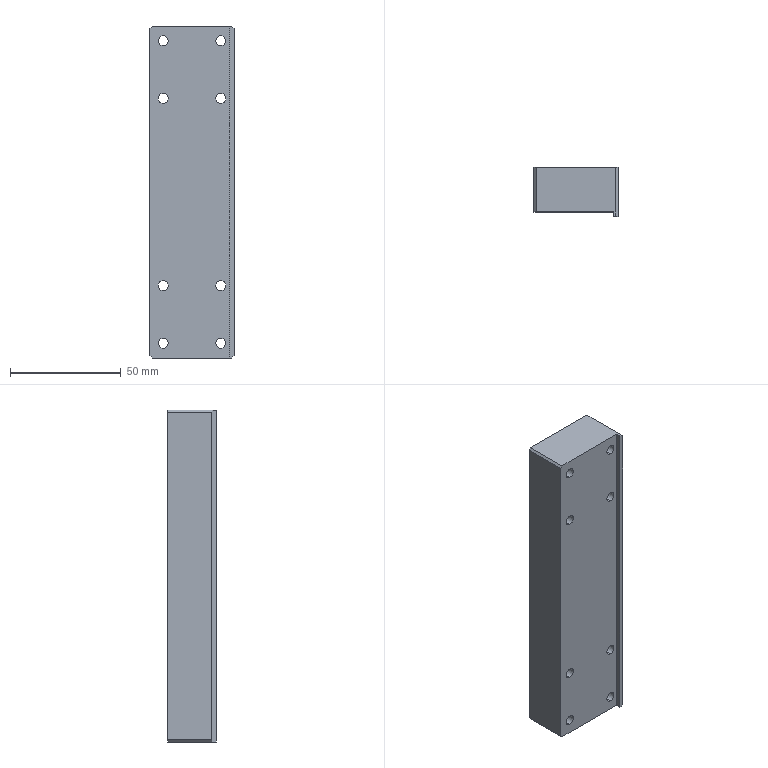Part | SolidWorks | features HoleWzd 4, Chamfer 1, Extrusion 1 | 1 solid | 92 faces | box 38 x 22 x 150 mm | volume 108993 mm3 | cylinder 52 | cone 20 | plane 20 | commonest cylinder face diameters 4.2 x18 4.5 x16 8 x16 5 x2